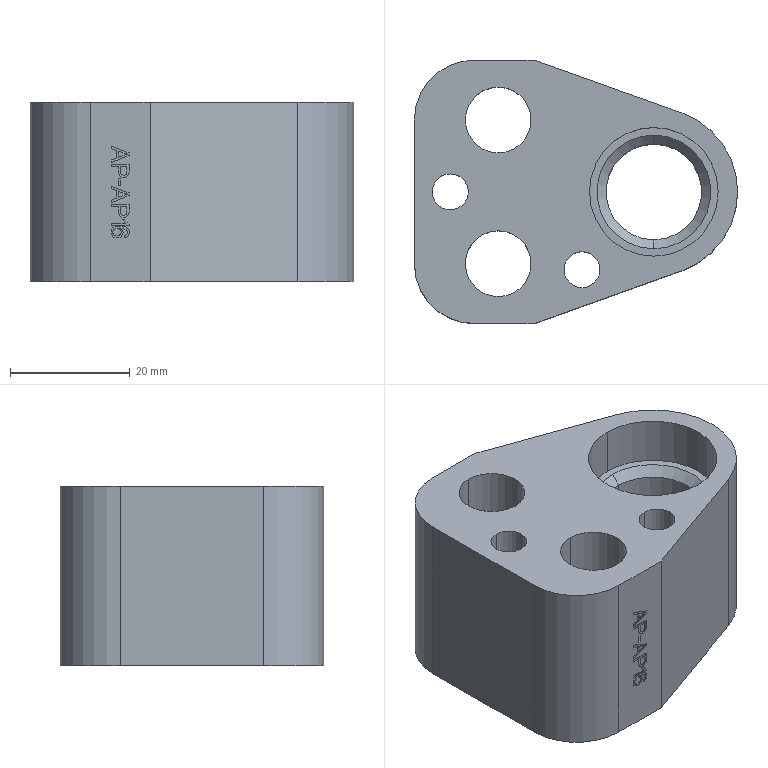Part | STEP file | gslz 2016.10.28-10_id610_x_t | 1 solid | 124 faces | box 54 x 44 x 30 mm | volume 37328 mm3 | plane 80 | cylinder 42 | cone 2 | commonest cylinder face diameters 6 x4 6.8 x4 8 x4 11 x4 17 x4 1.055 x2